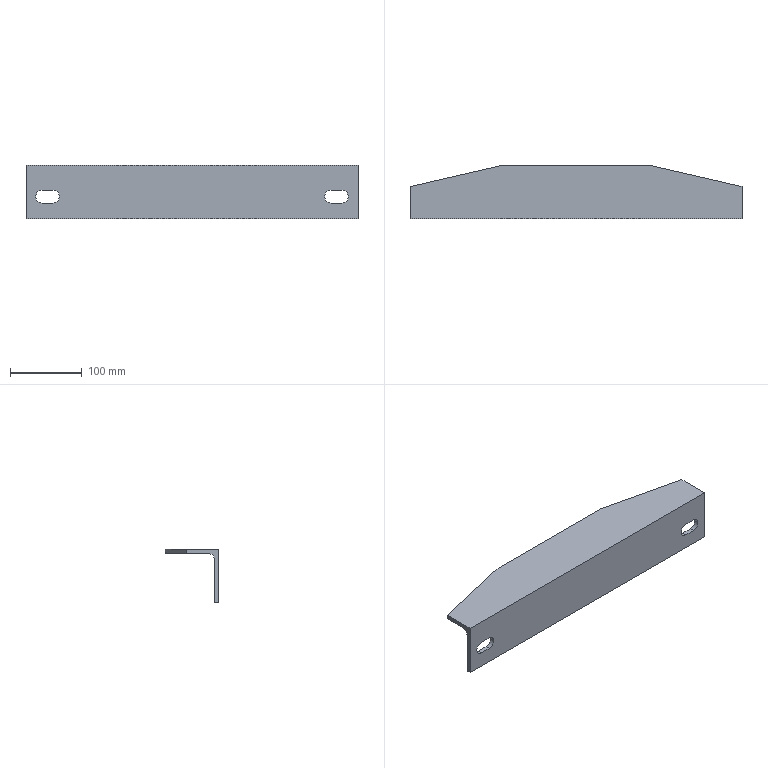Part | SolidWorks | features Chamfer 2, ICE 1, WeldMemberFeat 1, WeldmentFeature 1 | 1 solid | 21 faces | box 462 x 75 x 75 mm | volume 376932 mm3 | plane 14 | cylinder 7 | commonest cylinder face diameters 18 x5 4 x2
STEP:
#1=CARTESIAN_POINT('',(101.,75.,-4.));
#2=VERTEX_POINT('',#1);
#3=CARTESIAN_POINT('',(-101.,75.,-4.));
#4=VERTEX_POINT('',#3);
#5=CARTESIAN_POINT('',(231.,75.,-4.));
#6=DIRECTION('',(-1.,0.,0.));
#7=VECTOR('',#6,1000.);
#8=LINE('',#5,#7);
#9=EDGE_CURVE('',#2,#4,#8,.T.);
#10=ORIENTED_EDGE('',*,*,#9,.T.);
#11=CARTESIAN_POINT('',(-101.,75.,0.));
#12=VERTEX_POINT('',#11);
#13=CARTESIAN_POINT('',(-101.,75.,0.));
#14=DIRECTION('',(0.,0.,1.));
#15=VECTOR('',#14,1000.);
#16=LINE('',#13,#15);
#17=EDGE_CURVE('',#4,#12,#16,.T.);
#18=ORIENTED_EDGE('',*,*,#17,.T.);
#19=CARTESIAN_POINT('',(101.,75.,0.));
#20=VERTEX_POINT('',#19);
#21=CARTESIAN_POINT('',(231.,75.,0.));
#22=DIRECTION('',(-1.,0.,0.));
#23=VECTOR('',#22,1000.);
#24=LINE('',#21,#23);
#25=EDGE_CURVE('',#20,#12,#24,.T.);
#26=ORIENTED_EDGE('',*,*,#25,.F.);
#27=CARTESIAN_POINT('',(101.,75.,0.));
#28=DIRECTION('',(0.,0.,-1.));
#29=VECTOR('',#28,1000.);
#30=LINE('',#27,#29);
#31=EDGE_CURVE('',#20,#2,#30,.T.);
#32=ORIENTED_EDGE('',*,*,#31,.T.);
#33=EDGE_LOOP('',(#10,#18,#26,#32));
#34=FACE_OUTER_BOUND('',#33,.T.);
#35=CARTESIAN_POINT('',(231.,75.,0.));
#36=DIRECTION('',(0.,-1.,0.));
#37=DIRECTION('',(0.,0.,-1.));
#38=AXIS2_PLACEMENT_3D('',#35,#36,#37);
#39=PLANE('',#38);
#40=ADVANCED_FACE('',(#34),#39,.F.);
#41=ORIENTED_EDGE('',*,*,#25,.T.);
#42=CARTESIAN_POINT('',(-231.,45.,0.));
#43=VERTEX_POINT('',#42);
#44=CARTESIAN_POINT('',(-101.,75.,0.));
#45=DIRECTION('',(-0.9744,-0.2249,0.));
#46=VECTOR('',#45,1000.);
#47=LINE('',#44,#46);
#48=EDGE_CURVE('',#12,#43,#47,.T.);
#49=ORIENTED_EDGE('',*,*,#48,.T.);
#50=CARTESIAN_POINT('',(-231.,0.,0.));
#51=VERTEX_POINT('',#50);
#52=CARTESIAN_POINT('',(-231.,75.,0.));
#53=DIRECTION('',(0.,-1.,0.));
#54=VECTOR('',#53,1000.);
#55=LINE('',#52,#54);
#56=EDGE_CURVE('',#43,#51,#55,.T.);
#57=ORIENTED_EDGE('',*,*,#56,.T.);
#58=CARTESIAN_POINT('',(231.,0.,0.));
#59=VERTEX_POINT('',#58);
#60=CARTESIAN_POINT('',(231.,0.,0.));
#61=DIRECTION('',(-1.,0.,0.));
#62=VECTOR('',#61,1000.);
#63=LINE('',#60,#62);
#64=EDGE_CURVE('',#59,#51,#63,.T.);
#65=ORIENTED_EDGE('',*,*,#64,.F.);
#66=CARTESIAN_POINT('',(231.,45.,0.));
#67=VERTEX_POINT('',#66);
#68=CARTESIAN_POINT('',(231.,75.,0.));
#69=DIRECTION('',(0.,-1.,0.));
#70=VECTOR('',#69,1000.);
#71=LINE('',#68,#70);
#72=EDGE_CURVE('',#67,#59,#71,.T.);
#73=ORIENTED_EDGE('',*,*,#72,.F.);
#74=CARTESIAN_POINT('',(231.,45.,0.));
#75=DIRECTION('',(-0.9744,0.2249,0.));
#76=VECTOR('',#75,1000.);
#77=LINE('',#74,#76);
#78=EDGE_CURVE('',#67,#20,#77,.T.);
#79=ORIENTED_EDGE('',*,*,#78,.T.);
#80=EDGE_LOOP('',(#41,#49,#57,#65,#73,#79));
#81=FACE_OUTER_BOUND('',#80,.T.);
#82=CARTESIAN_POINT('',(231.,75.,0.));
#83=DIRECTION('',(0.,0.,-1.));
#84=DIRECTION('',(0.,1.,0.));
#85=AXIS2_PLACEMENT_3D('',#82,#83,#84);
#86=PLANE('',#85);
#87=ADVANCED_FACE('',(#81),#86,.F.);
#88=CARTESIAN_POINT('',(-208.5,0.,-53.));
#89=VERTEX_POINT('',#88);
#90=CARTESIAN_POINT('',(-193.5,0.,-53.));
#91=VERTEX_POINT('',#90);
#92=CARTESIAN_POINT('',(-208.5,0.,-53.));
#93=DIRECTION('',(1.,0.,0.));
#94=VECTOR('',#93,1000.);
#95=LINE('',#92,#94);
#96=EDGE_CURVE('',#89,#91,#95,.T.);
#97=ORIENTED_EDGE('',*,*,#96,.F.);
#98=CARTESIAN_POINT('',(-208.5,0.,-35.));
#99=VERTEX_POINT('',#98);
#100=CARTESIAN_POINT('',(-208.5,0.,-44.));
#101=DIRECTION('',(0.,-1.,0.));
#102=DIRECTION('',(0.,0.,1.));
#103=AXIS2_PLACEMENT_3D('',#100,#101,#102);
#104=CIRCLE('',#103,9.);
#105=EDGE_CURVE('',#99,#89,#104,.T.);
#106=ORIENTED_EDGE('',*,*,#105,.F.);
#107=CARTESIAN_POINT('',(-193.5,0.,-35.));
#108=VERTEX_POINT('',#107);
#109=CARTESIAN_POINT('',(-208.5,0.,-35.));
#110=DIRECTION('',(-1.,0.,0.));
#111=VECTOR('',#110,1000.);
#112=LINE('',#109,#111);
#113=EDGE_CURVE('',#108,#99,#112,.T.);
#114=ORIENTED_EDGE('',*,*,#113,.F.);
#115=CARTESIAN_POINT('',(-193.5,0.,-44.));
#116=DIRECTION('',(0.,-1.,0.));
#117=DIRECTION('',(0.,0.,1.));
#118=AXIS2_PLACEMENT_3D('',#115,#116,#117);
#119=CIRCLE('',#118,9.);
#120=EDGE_CURVE('',#91,#108,#119,.T.);
#121=ORIENTED_EDGE('',*,*,#120,.F.);
#122=EDGE_LOOP('',(#97,#106,#114,#121));
#123=FACE_BOUND('',#122,.T.);
#124=CARTESIAN_POINT('',(193.5,0.,-53.));
#125=VERTEX_POINT('',#124);
#126=CARTESIAN_POINT('',(208.5,0.,-53.));
#127=VERTEX_POINT('',#126);
#128=CARTESIAN_POINT('',(193.5,0.,-53.));
#129=DIRECTION('',(1.,0.,0.));
#130=VECTOR('',#129,1000.);
#131=LINE('',#128,#130);
#132=EDGE_CURVE('',#125,#127,#131,.T.);
#133=ORIENTED_EDGE('',*,*,#132,.F.);
#134=CARTESIAN_POINT('',(193.5,0.,-35.));
#135=VERTEX_POINT('',#134);
#136=CARTESIAN_POINT('',(193.5,0.,-44.));
#137=DIRECTION('',(0.,-1.,0.));
#138=DIRECTION('',(0.,0.,1.));
#139=AXIS2_PLACEMENT_3D('',#136,#137,#138);
#140=CIRCLE('',#139,9.);
#141=EDGE_CURVE('',#135,#125,#140,.T.);
#142=ORIENTED_EDGE('',*,*,#141,.F.);
#143=CARTESIAN_POINT('',(208.5,0.,-35.));
#144=VERTEX_POINT('',#143);
#145=CARTESIAN_POINT('',(193.5,0.,-35.));
#146=DIRECTION('',(-1.,0.,0.));
#147=VECTOR('',#146,1000.);
#148=LINE('',#145,#147);
#149=EDGE_CURVE('',#144,#135,#148,.T.);
#150=ORIENTED_EDGE('',*,*,#149,.F.);
#151=CARTESIAN_POINT('',(208.5,0.,-44.));
#152=DIRECTION('',(0.,-1.,0.));
#153=DIRECTION('',(0.,0.,1.));
#154=AXIS2_PLACEMENT_3D('',#151,#152,#153);
#155=CIRCLE('',#154,9.);
#156=EDGE_CURVE('',#127,#144,#155,.T.);
#157=ORIENTED_EDGE('',*,*,#156,.F.);
#158=EDGE_LOOP('',(#133,#142,#150,#157));
#159=FACE_BOUND('',#158,.T.);
#160=CARTESIAN_POINT('',(-231.,0.,-75.));
#161=VERTEX_POINT('',#160);
#162=CARTESIAN_POINT('',(-231.,0.,0.));
#163=DIRECTION('',(0.,0.,-1.));
#164=VECTOR('',#163,1000.);
#165=LINE('',#162,#164);
#166=EDGE_CURVE('',#51,#161,#165,.T.);
#167=ORIENTED_EDGE('',*,*,#166,.T.);
#168=CARTESIAN_POINT('',(231.,0.,-75.));
#169=VERTEX_POINT('',#168);
#170=CARTESIAN_POINT('',(231.,0.,-75.));
#171=DIRECTION('',(-1.,0.,0.));
#172=VECTOR('',#171,1000.);
#173=LINE('',#170,#172);
#174=EDGE_CURVE('',#169,#161,#173,.T.);
#175=ORIENTED_EDGE('',*,*,#174,.F.);
#176=CARTESIAN_POINT('',(231.,0.,0.));
#177=DIRECTION('',(0.,0.,-1.));
#178=VECTOR('',#177,1000.);
#179=LINE('',#176,#178);
#180=EDGE_CURVE('',#59,#169,#179,.T.);
#181=ORIENTED_EDGE('',*,*,#180,.F.);
#182=ORIENTED_EDGE('',*,*,#64,.T.);
#183=EDGE_LOOP('',(#167,#175,#181,#182));
#184=FACE_OUTER_BOUND('',#183,.T.);
#185=CARTESIAN_POINT('',(231.,0.,0.));
#186=DIRECTION('',(0.,1.,0.));
#187=DIRECTION('',(0.,0.,1.));
#188=AXIS2_PLACEMENT_3D('',#185,#186,#187);
#189=PLANE('',#188);
#190=ADVANCED_FACE('',(#123,#159,#184),#189,.F.);
#191=CARTESIAN_POINT('',(-231.,4.,-75.));
#192=VERTEX_POINT('',#191);
#193=CARTESIAN_POINT('',(-231.,0.,-75.));
#194=DIRECTION('',(0.,1.,0.));
#195=VECTOR('',#194,1000.);
#196=LINE('',#193,#195);
#197=EDGE_CURVE('',#161,#192,#196,.T.);
#198=ORIENTED_EDGE('',*,*,#197,.T.);
#199=CARTESIAN_POINT('',(231.,4.,-75.));
#200=VERTEX_POINT('',#199);
#201=CARTESIAN_POINT('',(231.,4.,-75.));
#202=DIRECTION('',(-1.,0.,0.));
#203=VECTOR('',#202,1000.);
#204=LINE('',#201,#203);
#205=EDGE_CURVE('',#200,#192,#204,.T.);
#206=ORIENTED_EDGE('',*,*,#205,.F.);
#207=CARTESIAN_POINT('',(231.,0.,-75.));
#208=DIRECTION('',(0.,1.,0.));
#209=VECTOR('',#208,1000.);
#210=LINE('',#207,#209);
#211=EDGE_CURVE('',#169,#200,#210,.T.);
#212=ORIENTED_EDGE('',*,*,#211,.F.);
#213=ORIENTED_EDGE('',*,*,#174,.T.);
#214=EDGE_LOOP('',(#198,#206,#212,#213));
#215=FACE_OUTER_BOUND('',#214,.T.);
#216=CARTESIAN_POINT('',(231.,0.,-75.));
#217=DIRECTION('',(0.,0.,1.));
#218=DIRECTION('',(0.,-1.,0.));
#219=AXIS2_PLACEMENT_3D('',#216,#217,#218);
#220=PLANE('',#219);
#221=ADVANCED_FACE('',(#215),#220,.F.);
#222=CARTESIAN_POINT('',(-231.,6.,-73.));
#223=VERTEX_POINT('',#222);
#224=CARTESIAN_POINT('',(-231.,4.,-73.));
#225=DIRECTION('',(1.,0.,0.));
#226=DIRECTION('',(0.,0.,-1.));
#227=AXIS2_PLACEMENT_3D('',#224,#225,#226);
#228=CIRCLE('',#227,2.);
#229=EDGE_CURVE('',#192,#223,#228,.T.);
#230=ORIENTED_EDGE('',*,*,#229,.T.);
#231=CARTESIAN_POINT('',(231.,6.,-73.));
#232=VERTEX_POINT('',#231);
#233=CARTESIAN_POINT('',(231.,6.,-73.));
#234=DIRECTION('',(-1.,0.,0.));
#235=VECTOR('',#234,1000.);
#236=LINE('',#233,#235);
#237=EDGE_CURVE('',#232,#223,#236,.T.);
#238=ORIENTED_EDGE('',*,*,#237,.F.);
#239=CARTESIAN_POINT('',(231.,4.,-73.));
#240=DIRECTION('',(1.,0.,0.));
#241=DIRECTION('',(0.,0.,-1.));
#242=AXIS2_PLACEMENT_3D('',#239,#240,#241);
#243=CIRCLE('',#242,2.);
#244=EDGE_CURVE('',#200,#232,#243,.T.);
#245=ORIENTED_EDGE('',*,*,#244,.F.);
#246=ORIENTED_EDGE('',*,*,#205,.T.);
#247=EDGE_LOOP('',(#230,#238,#245,#246));
#248=FACE_OUTER_BOUND('',#247,.T.);
#249=CARTESIAN_POINT('',(231.,4.,-73.));
#250=DIRECTION('',(-1.,0.,0.));
#251=DIRECTION('',(0.,0.,1.));
#252=AXIS2_PLACEMENT_3D('',#249,#250,#251);
#253=CYLINDRICAL_SURFACE('',#252,2.);
#254=ADVANCED_FACE('',(#248),#253,.T.);
#255=CARTESIAN_POINT('',(-208.5,6.,-35.));
#256=VERTEX_POINT('',#255);
#257=CARTESIAN_POINT('',(-193.5,6.,-35.));
#258=VERTEX_POINT('',#257);
#259=CARTESIAN_POINT('',(-208.5,6.,-35.));
#260=DIRECTION('',(1.,0.,0.));
#261=VECTOR('',#260,1000.);
#262=LINE('',#259,#261);
#263=EDGE_CURVE('',#256,#258,#262,.T.);
#264=ORIENTED_EDGE('',*,*,#263,.F.);
#265=CARTESIAN_POINT('',(-208.5,6.,-53.));
#266=VERTEX_POINT('',#265);
#267=CARTESIAN_POINT('',(-208.5,6.,-44.));
#268=DIRECTION('',(0.,1.,0.));
#269=DIRECTION('',(0.,0.,1.));
#270=AXIS2_PLACEMENT_3D('',#267,#268,#269);
#271=CIRCLE('',#270,9.);
#272=EDGE_CURVE('',#266,#256,#271,.T.);
#273=ORIENTED_EDGE('',*,*,#272,.F.);
#274=CARTESIAN_POINT('',(-193.5,6.,-53.));
#275=VERTEX_POINT('',#274);
#276=CARTESIAN_POINT('',(-208.5,6.,-53.));
#277=DIRECTION('',(-1.,0.,0.));
#278=VECTOR('',#277,1000.);
#279=LINE('',#276,#278);
#280=EDGE_CURVE('',#275,#266,#279,.T.);
#281=ORIENTED_EDGE('',*,*,#280,.F.);
#282=CARTESIAN_POINT('',(-193.5,6.,-44.));
#283=DIRECTION('',(0.,1.,0.));
#284=DIRECTION('',(0.,0.,1.));
#285=AXIS2_PLACEMENT_3D('',#282,#283,#284);
#286=CIRCLE('',#285,9.);
#287=EDGE_CURVE('',#258,#275,#286,.T.);
#288=ORIENTED_EDGE('',*,*,#287,.F.);
#289=EDGE_LOOP('',(#264,#273,#281,#288));
#290=FACE_BOUND('',#289,.T.);
#291=CARTESIAN_POINT('',(193.5,6.,-35.));
#292=VERTEX_POINT('',#291);
#293=CARTESIAN_POINT('',(208.5,6.,-35.));
#294=VERTEX_POINT('',#293);
#295=CARTESIAN_POINT('',(193.5,6.,-35.));
#296=DIRECTION('',(1.,0.,0.));
#297=VECTOR('',#296,1000.);
#298=LINE('',#295,#297);
#299=EDGE_CURVE('',#292,#294,#298,.T.);
#300=ORIENTED_EDGE('',*,*,#299,.F.);
#301=CARTESIAN_POINT('',(193.5,6.,-53.));
#302=VERTEX_POINT('',#301);
#303=CARTESIAN_POINT('',(193.5,6.,-44.));
#304=DIRECTION('',(0.,1.,0.));
#305=DIRECTION('',(0.,0.,1.));
#306=AXIS2_PLACEMENT_3D('',#303,#304,#305);
#307=CIRCLE('',#306,9.);
#308=EDGE_CURVE('',#302,#292,#307,.T.);
#309=ORIENTED_EDGE('',*,*,#308,.F.);
#310=CARTESIAN_POINT('',(208.5,6.,-53.));
#311=VERTEX_POINT('',#310);
#312=CARTESIAN_POINT('',(193.5,6.,-53.));
#313=DIRECTION('',(-1.,0.,0.));
#314=VECTOR('',#313,1000.);
#315=LINE('',#312,#314);
#316=EDGE_CURVE('',#311,#302,#315,.T.);
#317=ORIENTED_EDGE('',*,*,#316,.F.);
#318=CARTESIAN_POINT('',(208.5,6.,-44.));
#319=DIRECTION('',(0.,1.,0.));
#320=DIRECTION('',(0.,0.,1.));
#321=AXIS2_PLACEMENT_3D('',#318,#319,#320);
#322=CIRCLE('',#321,9.);
#323=EDGE_CURVE('',#294,#311,#322,.T.);
#324=ORIENTED_EDGE('',*,*,#323,.F.);
#325=EDGE_LOOP('',(#300,#309,#317,#324));
#326=FACE_BOUND('',#325,.T.);
#327=CARTESIAN_POINT('',(-231.,6.,-15.));
#328=VERTEX_POINT('',#327);
#329=CARTESIAN_POINT('',(-231.,6.,-15.));
#330=DIRECTION('',(0.,0.,1.));
#331=VECTOR('',#330,1000.);
#332=LINE('',#329,#331);
#333=EDGE_CURVE('',#223,#328,#332,.T.);
#334=ORIENTED_EDGE('',*,*,#333,.T.);
#335=CARTESIAN_POINT('',(231.,6.,-15.));
#336=VERTEX_POINT('',#335);
#337=CARTESIAN_POINT('',(231.,6.,-15.));
#338=DIRECTION('',(-1.,0.,0.));
#339=VECTOR('',#338,1000.);
#340=LINE('',#337,#339);
#341=EDGE_CURVE('',#336,#328,#340,.T.);
#342=ORIENTED_EDGE('',*,*,#341,.F.);
#343=CARTESIAN_POINT('',(231.,6.,-15.));
#344=DIRECTION('',(0.,0.,1.));
#345=VECTOR('',#344,1000.);
#346=LINE('',#343,#345);
#347=EDGE_CURVE('',#232,#336,#346,.T.);
#348=ORIENTED_EDGE('',*,*,#347,.F.);
#349=ORIENTED_EDGE('',*,*,#237,.T.);
#350=EDGE_LOOP('',(#334,#342,#348,#349));
#351=FACE_OUTER_BOUND('',#350,.T.);
#352=CARTESIAN_POINT('',(231.,6.,-15.));
#353=DIRECTION('',(0.,-1.,0.));
#354=DIRECTION('',(0.,0.,-1.));
#355=AXIS2_PLACEMENT_3D('',#352,#353,#354);
#356=PLANE('',#355);
#357=ADVANCED_FACE('',(#290,#326,#351),#356,.F.);
#358=CARTESIAN_POINT('',(-231.,15.,-6.));
#359=VERTEX_POINT('',#358);
#360=CARTESIAN_POINT('',(-231.,15.,-15.));
#361=DIRECTION('',(-1.,0.,0.));
#362=DIRECTION('',(0.,0.,-1.));
#363=AXIS2_PLACEMENT_3D('',#360,#361,#362);
#364=CIRCLE('',#363,9.);
#365=EDGE_CURVE('',#328,#359,#364,.T.);
#366=ORIENTED_EDGE('',*,*,#365,.T.);
#367=CARTESIAN_POINT('',(231.,15.,-6.));
#368=VERTEX_POINT('',#367);
#369=CARTESIAN_POINT('',(231.,15.,-6.));
#370=DIRECTION('',(-1.,0.,0.));
#371=VECTOR('',#370,1000.);
#372=LINE('',#369,#371);
#373=EDGE_CURVE('',#368,#359,#372,.T.);
#374=ORIENTED_EDGE('',*,*,#373,.F.);
#375=CARTESIAN_POINT('',(231.,15.,-15.));
#376=DIRECTION('',(-1.,0.,0.));
#377=DIRECTION('',(0.,0.,-1.));
#378=AXIS2_PLACEMENT_3D('',#375,#376,#377);
#379=CIRCLE('',#378,9.);
#380=EDGE_CURVE('',#336,#368,#379,.T.);
#381=ORIENTED_EDGE('',*,*,#380,.F.);
#382=ORIENTED_EDGE('',*,*,#341,.T.);
#383=EDGE_LOOP('',(#366,#374,#381,#382));
#384=FACE_OUTER_BOUND('',#383,.T.);
#385=CARTESIAN_POINT('',(231.,15.,-15.));
#386=DIRECTION('',(-1.,0.,0.));
#387=DIRECTION('',(0.,0.,1.));
#388=AXIS2_PLACEMENT_3D('',#385,#386,#387);
#389=CYLINDRICAL_SURFACE('',#388,9.);
#390=ADVANCED_FACE('',(#384),#389,.F.);
#391=CARTESIAN_POINT('',(-231.,45.,-6.));
#392=VERTEX_POINT('',#391);
#393=CARTESIAN_POINT('',(-231.,73.,-6.));
#394=DIRECTION('',(0.,1.,0.));
#395=VECTOR('',#394,1000.);
#396=LINE('',#393,#395);
#397=EDGE_CURVE('',#359,#392,#396,.T.);
#398=ORIENTED_EDGE('',*,*,#397,.T.);
#399=CARTESIAN_POINT('',(-109.667,73.,-6.));
#400=VERTEX_POINT('',#399);
#401=CARTESIAN_POINT('',(-101.,75.,-6.));
#402=DIRECTION('',(0.9744,0.2249,0.));
#403=VECTOR('',#402,1000.);
#404=LINE('',#401,#403);
#405=EDGE_CURVE('',#392,#400,#404,.T.);
#406=ORIENTED_EDGE('',*,*,#405,.T.);
#407=CARTESIAN_POINT('',(109.667,73.,-6.));
#408=VERTEX_POINT('',#407);
#409=CARTESIAN_POINT('',(231.,73.,-6.));
#410=DIRECTION('',(-1.,0.,0.));
#411=VECTOR('',#410,1000.);
#412=LINE('',#409,#411);
#413=EDGE_CURVE('',#408,#400,#412,.T.);
#414=ORIENTED_EDGE('',*,*,#413,.F.);
#415=CARTESIAN_POINT('',(231.,45.,-6.));
#416=VERTEX_POINT('',#415);
#417=CARTESIAN_POINT('',(231.,45.,-6.));
#418=DIRECTION('',(0.9744,-0.2249,0.));
#419=VECTOR('',#418,1000.);
#420=LINE('',#417,#419);
#421=EDGE_CURVE('',#408,#416,#420,.T.);
#422=ORIENTED_EDGE('',*,*,#421,.T.);
#423=CARTESIAN_POINT('',(231.,73.,-6.));
#424=DIRECTION('',(0.,1.,0.));
#425=VECTOR('',#424,1000.);
#426=LINE('',#423,#425);
#427=EDGE_CURVE('',#368,#416,#426,.T.);
#428=ORIENTED_EDGE('',*,*,#427,.F.);
#429=ORIENTED_EDGE('',*,*,#373,.T.);
#430=EDGE_LOOP('',(#398,#406,#414,#422,#428,#429));
#431=FACE_OUTER_BOUND('',#430,.T.);
#432=CARTESIAN_POINT('',(231.,73.,-6.));
#433=DIRECTION('',(0.,0.,1.));
#434=DIRECTION('',(0.,-1.,0.));
#435=AXIS2_PLACEMENT_3D('',#432,#433,#434);
#436=PLANE('',#435);
#437=ADVANCED_FACE('',(#431),#436,.F.);
#438=ORIENTED_EDGE('',*,*,#413,.T.);
#439=CARTESIAN_POINT('',(-109.667,73.,-6.));
#440=CARTESIAN_POINT('',(-104.59,74.172,-6.));
#441=CARTESIAN_POINT('',(-101.,75.,-5.172));
#442=CARTESIAN_POINT('',(-101.,75.,-4.));
#443=(BOUNDED_CURVE()B_SPLINE_CURVE(3,(#439,#440,#441,#442),.UNSPECIFIED.,.F.,.F.)B_SPLINE_CURVE_WITH_KNOTS((4,4),(1.571,3.142),.UNSPECIFIED.)CURVE()GEOMETRIC_REPRESENTATION_ITEM()RATIONAL_B_SPLINE_CURVE((1.,0.8047,0.8047,1.))REPRESENTATION_ITEM(''));
#444=EDGE_CURVE('',#400,#4,#443,.T.);
#445=ORIENTED_EDGE('',*,*,#444,.T.);
#446=ORIENTED_EDGE('',*,*,#9,.F.);
#447=CARTESIAN_POINT('',(101.,75.,-4.));
#448=CARTESIAN_POINT('',(101.,75.,-5.172));
#449=CARTESIAN_POINT('',(104.59,74.172,-6.));
#450=CARTESIAN_POINT('',(109.667,73.,-6.));
#451=(BOUNDED_CURVE()B_SPLINE_CURVE(3,(#447,#448,#449,#450),.UNSPECIFIED.,.F.,.F.)B_SPLINE_CURVE_WITH_KNOTS((4,4),(0.,1.571),.UNSPECIFIED.)CURVE()GEOMETRIC_REPRESENTATION_ITEM()RATIONAL_B_SPLINE_CURVE((1.,0.8047,0.8047,1.))REPRESENTATION_ITEM(''));
#452=EDGE_CURVE('',#2,#408,#451,.T.);
#453=ORIENTED_EDGE('',*,*,#452,.T.);
#454=EDGE_LOOP('',(#438,#445,#446,#453));
#455=FACE_OUTER_BOUND('',#454,.T.);
#456=CARTESIAN_POINT('',(231.,73.,-4.));
#457=DIRECTION('',(-1.,0.,0.));
#458=DIRECTION('',(0.,0.,1.));
#459=AXIS2_PLACEMENT_3D('',#456,#457,#458);
#460=CYLINDRICAL_SURFACE('',#459,2.);
#461=ADVANCED_FACE('',(#455),#460,.T.);
#462=ORIENTED_EDGE('',*,*,#427,.T.);
#463=CARTESIAN_POINT('',(231.,45.,-4.));
#464=DIRECTION('',(0.,0.,1.));
#465=VECTOR('',#464,1000.);
#466=LINE('',#463,#465);
#467=EDGE_CURVE('',#416,#67,#466,.T.);
#468=ORIENTED_EDGE('',*,*,#467,.T.);
#469=ORIENTED_EDGE('',*,*,#72,.T.);
#470=ORIENTED_EDGE('',*,*,#180,.T.);
#471=ORIENTED_EDGE('',*,*,#211,.T.);
#472=ORIENTED_EDGE('',*,*,#244,.T.);
#473=ORIENTED_EDGE('',*,*,#347,.T.);
#474=ORIENTED_EDGE('',*,*,#380,.T.);
#475=EDGE_LOOP('',(#462,#468,#469,#470,#471,#472,#473,#474));
#476=FACE_OUTER_BOUND('',#475,.T.);
#477=CARTESIAN_POINT('',(231.,73.,-4.));
#478=DIRECTION('',(-1.,0.,0.));
#479=DIRECTION('',(0.,0.,1.));
#480=AXIS2_PLACEMENT_3D('',#477,#478,#479);
#481=PLANE('',#480);
#482=ADVANCED_FACE('',(#476),#481,.F.);
#483=ORIENTED_EDGE('',*,*,#56,.F.);
#484=CARTESIAN_POINT('',(-231.,45.,-4.));
#485=DIRECTION('',(0.,0.,-1.));
#486=VECTOR('',#485,1000.);
#487=LINE('',#484,#486);
#488=EDGE_CURVE('',#43,#392,#487,.T.);
#489=ORIENTED_EDGE('',*,*,#488,.T.);
#490=ORIENTED_EDGE('',*,*,#397,.F.);
#491=ORIENTED_EDGE('',*,*,#365,.F.);
#492=ORIENTED_EDGE('',*,*,#333,.F.);
#493=ORIENTED_EDGE('',*,*,#229,.F.);
#494=ORIENTED_EDGE('',*,*,#197,.F.);
#495=ORIENTED_EDGE('',*,*,#166,.F.);
#496=EDGE_LOOP('',(#483,#489,#490,#491,#492,#493,#494,#495));
#497=FACE_OUTER_BOUND('',#496,.T.);
#498=CARTESIAN_POINT('',(-231.,73.,-4.));
#499=DIRECTION('',(-1.,0.,0.));
#500=DIRECTION('',(0.,0.,1.));
#501=AXIS2_PLACEMENT_3D('',#498,#499,#500);
#502=PLANE('',#501);
#503=ADVANCED_FACE('',(#497),#502,.T.);
#504=ORIENTED_EDGE('',*,*,#141,.T.);
#505=CARTESIAN_POINT('',(193.5,-0.001,-53.));
#506=DIRECTION('',(0.,1.,0.));
#507=VECTOR('',#506,1000.);
#508=LINE('',#505,#507);
#509=EDGE_CURVE('',#125,#302,#508,.T.);
#510=ORIENTED_EDGE('',*,*,#509,.T.);
#511=ORIENTED_EDGE('',*,*,#308,.T.);
#512=CARTESIAN_POINT('',(193.5,-0.001,-35.));
#513=DIRECTION('',(0.,1.,0.));
#514=VECTOR('',#513,1000.);
#515=LINE('',#512,#514);
#516=EDGE_CURVE('',#135,#292,#515,.T.);
#517=ORIENTED_EDGE('',*,*,#516,.F.);
#518=EDGE_LOOP('',(#504,#510,#511,#517));
#519=FACE_OUTER_BOUND('',#518,.T.);
#520=CARTESIAN_POINT('',(193.5,-0.001,-44.));
#521=DIRECTION('',(0.,1.,0.));
#522=DIRECTION('',(0.,0.,1.));
#523=AXIS2_PLACEMENT_3D('',#520,#521,#522);
#524=CYLINDRICAL_SURFACE('',#523,9.);
#525=ADVANCED_FACE('',(#519),#524,.F.);
#526=ORIENTED_EDGE('',*,*,#132,.T.);
#527=CARTESIAN_POINT('',(208.5,-0.001,-53.));
#528=DIRECTION('',(0.,1.,0.));
#529=VECTOR('',#528,1000.);
#530=LINE('',#527,#529);
#531=EDGE_CURVE('',#127,#311,#530,.T.);
#532=ORIENTED_EDGE('',*,*,#531,.T.);
#533=ORIENTED_EDGE('',*,*,#316,.T.);
#534=ORIENTED_EDGE('',*,*,#509,.F.);
#535=EDGE_LOOP('',(#526,#532,#533,#534));
#536=FACE_OUTER_BOUND('',#535,.T.);
#537=CARTESIAN_POINT('',(193.5,-0.001,-53.));
#538=DIRECTION('',(0.,0.,-1.));
#539=DIRECTION('',(0.,1.,0.));
#540=AXIS2_PLACEMENT_3D('',#537,#538,#539);
#541=PLANE('',#540);
#542=ADVANCED_FACE('',(#536),#541,.F.);
#543=ORIENTED_EDGE('',*,*,#156,.T.);
#544=CARTESIAN_POINT('',(208.5,-0.001,-35.));
#545=DIRECTION('',(0.,1.,0.));
#546=VECTOR('',#545,1000.);
#547=LINE('',#544,#546);
#548=EDGE_CURVE('',#144,#294,#547,.T.);
#549=ORIENTED_EDGE('',*,*,#548,.T.);
#550=ORIENTED_EDGE('',*,*,#323,.T.);
#551=ORIENTED_EDGE('',*,*,#531,.F.);
#552=EDGE_LOOP('',(#543,#549,#550,#551));
#553=FACE_OUTER_BOUND('',#552,.T.);
#554=CARTESIAN_POINT('',(208.5,-0.001,-44.));
#555=DIRECTION('',(0.,1.,0.));
#556=DIRECTION('',(0.,0.,1.));
#557=AXIS2_PLACEMENT_3D('',#554,#555,#556);
#558=CYLINDRICAL_SURFACE('',#557,9.);
#559=ADVANCED_FACE('',(#553),#558,.F.);
#560=ORIENTED_EDGE('',*,*,#149,.T.);
#561=ORIENTED_EDGE('',*,*,#516,.T.);
#562=ORIENTED_EDGE('',*,*,#299,.T.);
#563=ORIENTED_EDGE('',*,*,#548,.F.);
#564=EDGE_LOOP('',(#560,#561,#562,#563));
#565=FACE_OUTER_BOUND('',#564,.T.);
#566=CARTESIAN_POINT('',(193.5,-0.001,-35.));
#567=DIRECTION('',(0.,0.,1.));
#568=DIRECTION('',(1.,0.,0.));
#569=AXIS2_PLACEMENT_3D('',#566,#567,#568);
#570=PLANE('',#569);
#571=ADVANCED_FACE('',(#565),#570,.F.);
#572=ORIENTED_EDGE('',*,*,#105,.T.);
#573=CARTESIAN_POINT('',(-208.5,-0.001,-53.));
#574=DIRECTION('',(0.,1.,0.));
#575=VECTOR('',#574,1000.);
#576=LINE('',#573,#575);
#577=EDGE_CURVE('',#89,#266,#576,.T.);
#578=ORIENTED_EDGE('',*,*,#577,.T.);
#579=ORIENTED_EDGE('',*,*,#272,.T.);
#580=CARTESIAN_POINT('',(-208.5,-0.001,-35.));
#581=DIRECTION('',(0.,1.,0.));
#582=VECTOR('',#581,1000.);
#583=LINE('',#580,#582);
#584=EDGE_CURVE('',#99,#256,#583,.T.);
#585=ORIENTED_EDGE('',*,*,#584,.F.);
#586=EDGE_LOOP('',(#572,#578,#579,#585));
#587=FACE_OUTER_BOUND('',#586,.T.);
#588=CARTESIAN_POINT('',(-208.5,-0.001,-44.));
#589=DIRECTION('',(0.,1.,0.));
#590=DIRECTION('',(0.,0.,1.));
#591=AXIS2_PLACEMENT_3D('',#588,#589,#590);
#592=CYLINDRICAL_SURFACE('',#591,9.);
#593=ADVANCED_FACE('',(#587),#592,.F.);
#594=ORIENTED_EDGE('',*,*,#96,.T.);
#595=CARTESIAN_POINT('',(-193.5,-0.001,-53.));
#596=DIRECTION('',(0.,1.,0.));
#597=VECTOR('',#596,1000.);
#598=LINE('',#595,#597);
#599=EDGE_CURVE('',#91,#275,#598,.T.);
#600=ORIENTED_EDGE('',*,*,#599,.T.);
#601=ORIENTED_EDGE('',*,*,#280,.T.);
#602=ORIENTED_EDGE('',*,*,#577,.F.);
#603=EDGE_LOOP('',(#594,#600,#601,#602));
#604=FACE_OUTER_BOUND('',#603,.T.);
#605=CARTESIAN_POINT('',(-208.5,-0.001,-53.));
#606=DIRECTION('',(0.,0.,-1.));
#607=DIRECTION('',(-1.,0.,0.));
#608=AXIS2_PLACEMENT_3D('',#605,#606,#607);
#609=PLANE('',#608);
#610=ADVANCED_FACE('',(#604),#609,.F.);
#611=ORIENTED_EDGE('',*,*,#120,.T.);
#612=CARTESIAN_POINT('',(-193.5,-0.001,-35.));
#613=DIRECTION('',(0.,1.,0.));
#614=VECTOR('',#613,1000.);
#615=LINE('',#612,#614);
#616=EDGE_CURVE('',#108,#258,#615,.T.);
#617=ORIENTED_EDGE('',*,*,#616,.T.);
#618=ORIENTED_EDGE('',*,*,#287,.T.);
#619=ORIENTED_EDGE('',*,*,#599,.F.);
#620=EDGE_LOOP('',(#611,#617,#618,#619));
#621=FACE_OUTER_BOUND('',#620,.T.);
#622=CARTESIAN_POINT('',(-193.5,-0.001,-44.));
#623=DIRECTION('',(0.,1.,0.));
#624=DIRECTION('',(0.,0.,1.));
#625=AXIS2_PLACEMENT_3D('',#622,#623,#624);
#626=CYLINDRICAL_SURFACE('',#625,9.);
#627=ADVANCED_FACE('',(#621),#626,.F.);
#628=ORIENTED_EDGE('',*,*,#113,.T.);
#629=ORIENTED_EDGE('',*,*,#584,.T.);
#630=ORIENTED_EDGE('',*,*,#263,.T.);
#631=ORIENTED_EDGE('',*,*,#616,.F.);
#632=EDGE_LOOP('',(#628,#629,#630,#631));
#633=FACE_OUTER_BOUND('',#632,.T.);
#634=CARTESIAN_POINT('',(-208.5,-0.001,-35.));
#635=DIRECTION('',(0.,0.,1.));
#636=DIRECTION('',(0.,-1.,0.));
#637=AXIS2_PLACEMENT_3D('',#634,#635,#636);
#638=PLANE('',#637);
#639=ADVANCED_FACE('',(#633),#638,.F.);
#640=ORIENTED_EDGE('',*,*,#452,.F.);
#641=ORIENTED_EDGE('',*,*,#31,.F.);
#642=ORIENTED_EDGE('',*,*,#78,.F.);
#643=ORIENTED_EDGE('',*,*,#467,.F.);
#644=ORIENTED_EDGE('',*,*,#421,.F.);
#645=EDGE_LOOP('',(#640,#641,#642,#643,#644));
#646=FACE_OUTER_BOUND('',#645,.T.);
#647=CARTESIAN_POINT('',(231.,45.,-4.));
#648=DIRECTION('',(-0.2249,-0.9744,0.));
#649=DIRECTION('',(0.,0.,1.));
#650=AXIS2_PLACEMENT_3D('',#647,#648,#649);
#651=PLANE('',#650);
#652=ADVANCED_FACE('',(#646),#651,.F.);
#653=ORIENTED_EDGE('',*,*,#405,.F.);
#654=ORIENTED_EDGE('',*,*,#488,.F.);
#655=ORIENTED_EDGE('',*,*,#48,.F.);
#656=ORIENTED_EDGE('',*,*,#17,.F.);
#657=ORIENTED_EDGE('',*,*,#444,.F.);
#658=EDGE_LOOP('',(#653,#654,#655,#656,#657));
#659=FACE_OUTER_BOUND('',#658,.T.);
#660=CARTESIAN_POINT('',(-101.,75.,0.));
#661=DIRECTION('',(-0.2249,0.9744,0.));
#662=DIRECTION('',(0.,0.,-1.));
#663=AXIS2_PLACEMENT_3D('',#660,#661,#662);
#664=PLANE('',#663);
#665=ADVANCED_FACE('',(#659),#664,.T.);
#666=CLOSED_SHELL('',(#40,#87,#190,#221,#254,#357,#390,#437,#461,#482,#503,#525,#542,#559,#571,#593,#610,#627,#639,#652,#665));
#667=MANIFOLD_SOLID_BREP('',#666);
#668=CARTESIAN_POINT('',(0.,0.,0.));
#669=DIRECTION('',(0.,0.,1.));
#670=DIRECTION('',(1.,0.,0.));
#671=AXIS2_PLACEMENT_3D('',#668,#669,#670);
#672=(LENGTH_UNIT()NAMED_UNIT(*)SI_UNIT(.MILLI.,.METRE.));
#673=UNCERTAINTY_MEASURE_WITH_UNIT(LENGTH_MEASURE(0.00001),#672,'','');
#674=(NAMED_UNIT(*)PLANE_ANGLE_UNIT()SI_UNIT($,.RADIAN.));
#675=(NAMED_UNIT(*)SI_UNIT($,.STERADIAN.)SOLID_ANGLE_UNIT());
#676=(GEOMETRIC_REPRESENTATION_CONTEXT(3)GLOBAL_UNCERTAINTY_ASSIGNED_CONTEXT((#673))GLOBAL_UNIT_ASSIGNED_CONTEXT((#672,#674,#675))REPRESENTATION_CONTEXT('',''));
#677=ADVANCED_BREP_SHAPE_REPRESENTATION('',(#667,#671),#676);